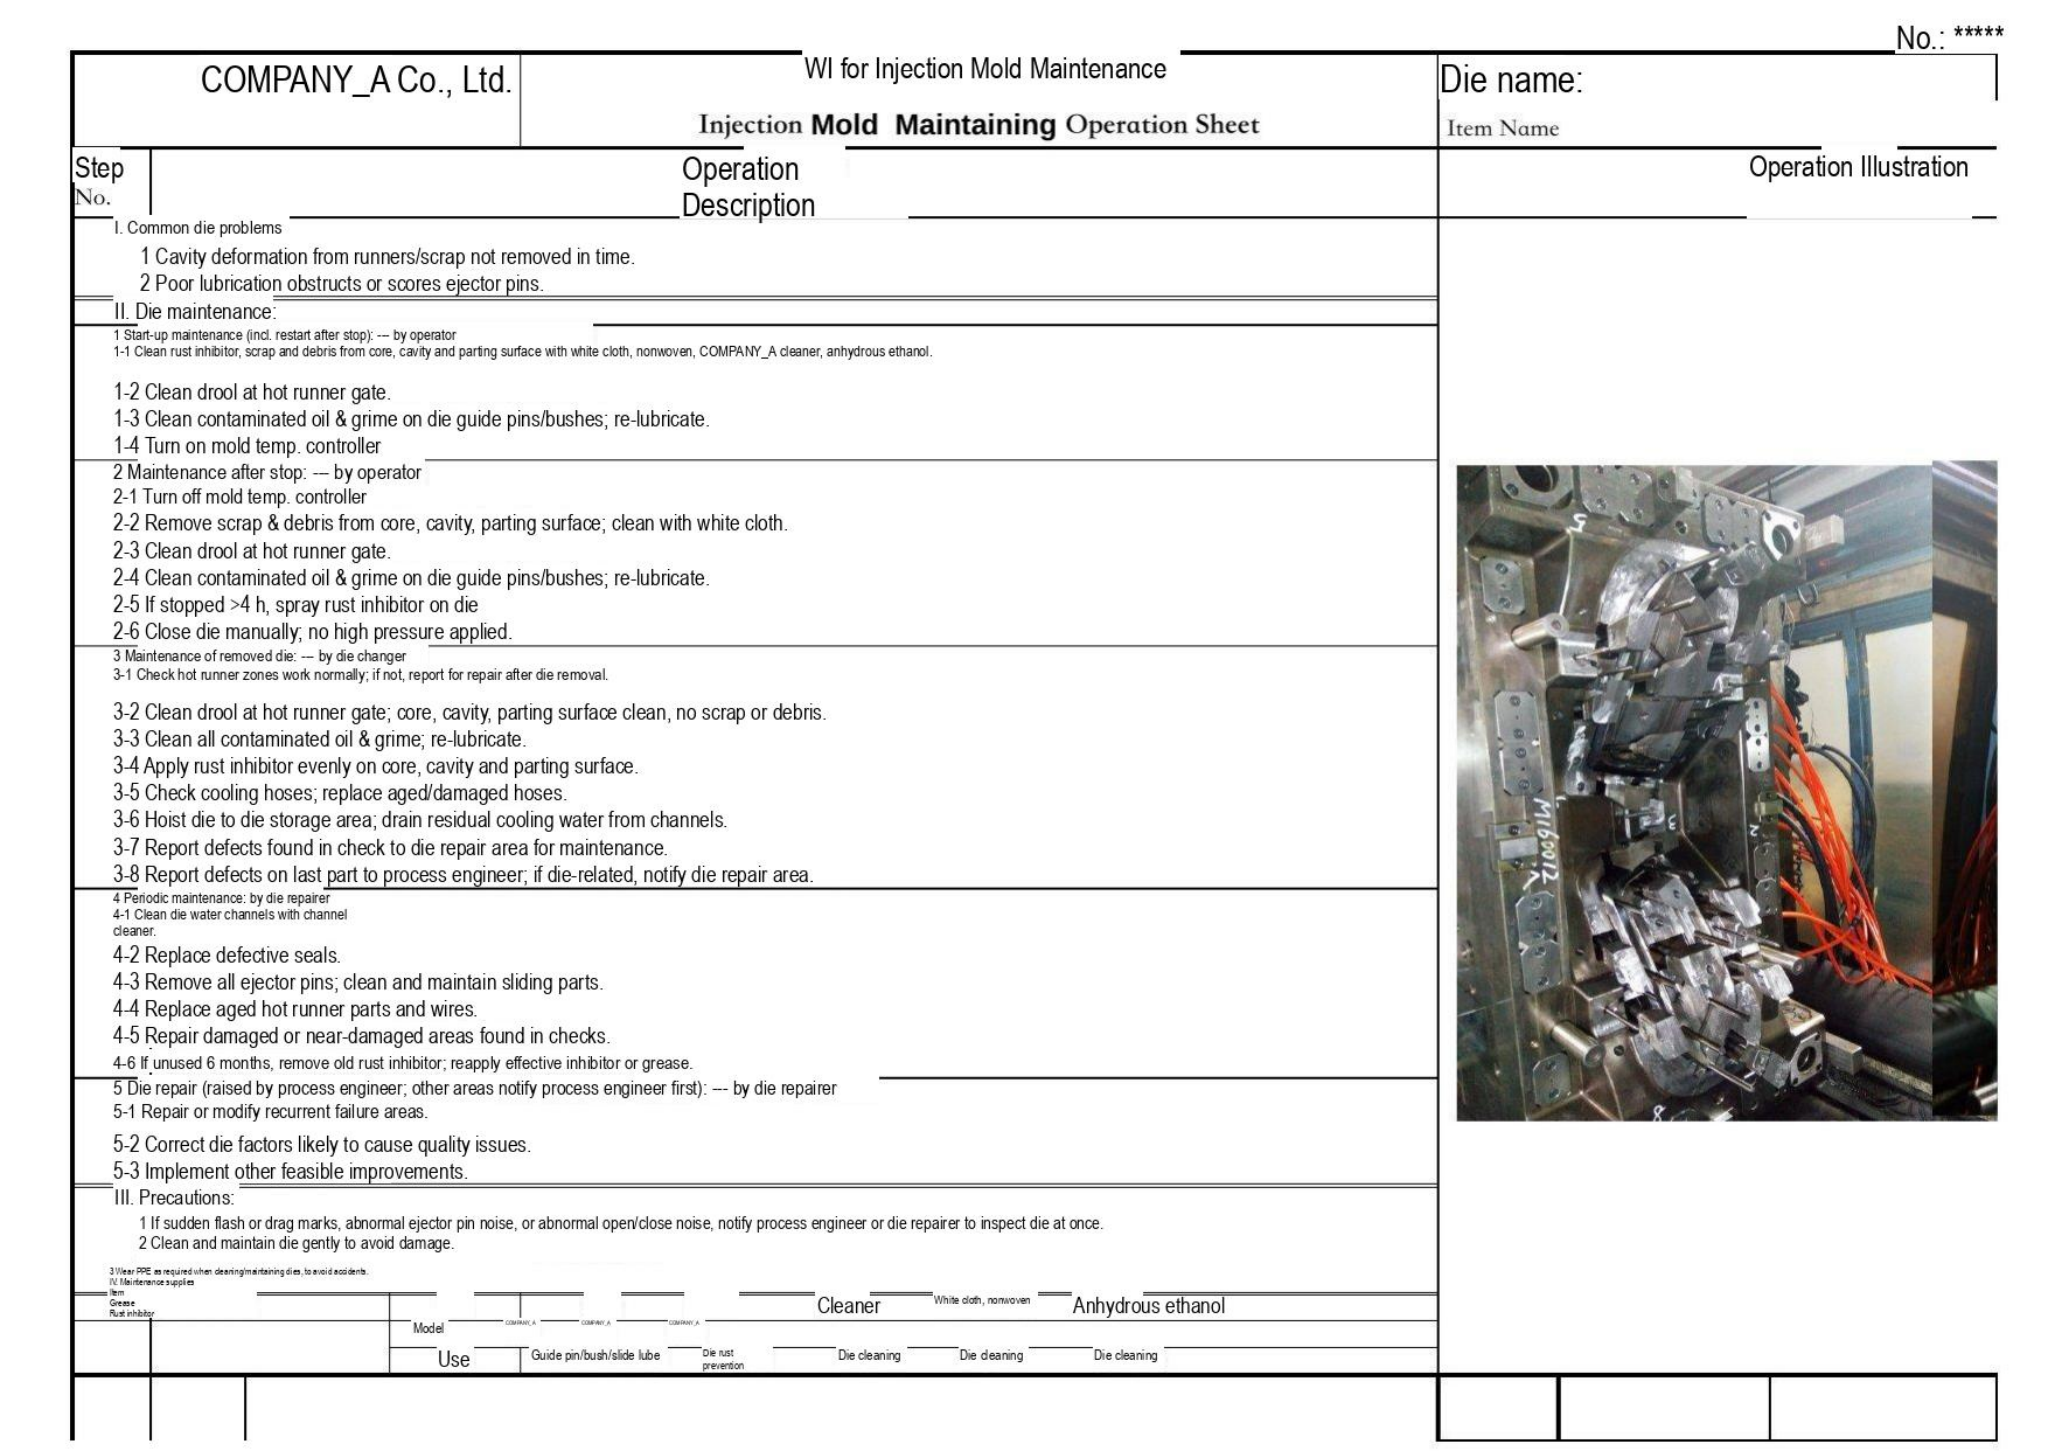No.: *****

COMPANY_A Co., Ltd.

WI for Injection Mold Maintenance

Injection Mold Maintaining Operation Sheet

Die name:

Item Name

Step No.

Operation Description

Operation Illustration

I. Common die problems

1 Cavity deformation from runners/scrap not removed in time.

2 Poor lubrication obstructs or scores ejector pins.

II. Die maintenance:

1 Start-up maintenance (incl. restart after stop): --- by operator

1-1 Clean rust inhibitor, scrap and debris from core, cavity and parting surface with white cloth, nonwoven, COMPANY_A cleaner, anhydrous ethanol.

1-2 Clean drool at hot runner gate.

1-3 Clean contaminated oil & grime on die guide pins/bushes; re-lubricate.

1-4 Turn on mold temp. controller

2 Maintenance after stop: --- by operator

2-1 Turn off mold temp. controller

2-2 Remove scrap & debris from core, cavity, parting surface; clean with white cloth.

2-3 Clean drool at hot runner gate.

2-4 Clean contaminated oil & grime on die guide pins/bushes; re-lubricate.

2-5 If stopped >4 h, spray rust inhibitor on die

2-6 Close die manually; no high pressure applied.

3 Maintenance of removed die: --- by die changer

3-1 Check hot runner zones work normally; if not, report for repair after die removal.

3-2 Clean drool at hot runner gate; core, cavity, parting surface clean, no scrap or debris.

3-3 Clean all contaminated oil & grime; re-lubricate.

3-4 Apply rust inhibitor evenly on core, cavity and parting surface.

3-5 Check cooling hoses; replace aged/damaged hoses.

3-6 Hoist die to die storage area; drain residual cooling water from channels.

3-7 Report defects found in check to die repair area for maintenance.

3-8 Report defects on last part to process engineer; if die-related, notify die repair area.

4 Periodic maintenance: by die repairer

4-1 Clean die water channels with channel cleaner.

4-2 Replace defective seals.

4-3 Remove all ejector pins; clean and maintain sliding parts.

4-4 Replace aged hot runner parts and wires.

4-5 Repair damaged or near-damaged areas found in checks.

4-6 If unused 6 months, remove old rust inhibitor; reapply effective inhibitor or grease.

5 Die repair (raised by process engineer; other areas notify process engineer first): --- by die repairer

5-1 Repair or modify recurrent failure areas.

5-2 Correct die factors likely to cause quality issues.

5-3 Implement other feasible improvements.

III. Precautions:

1 If sudden flash or drag marks, abnormal ejector pin noise, or abnormal open/close noise, notify process engineer or die repairer to inspect die at once.

2 Clean and maintain die gently to avoid damage.

3 Wear PPE as required when cleaning/maintaining dies, to avoid accidents.

IV. Maintenance supplies

| Item | Grease | Rust inhibitor | Cleaner | White cloth, nonwoven | Anhydrous ethanol |
|---|---|---|---|---|---|
| Model | COMPANY_A | COMPANY_A | COMPANY_A | | |
| Use | Guide pin/bush/slide lube | Die rust prevention | Die cleaning | Die cleaning | Die cleaning |

M160012
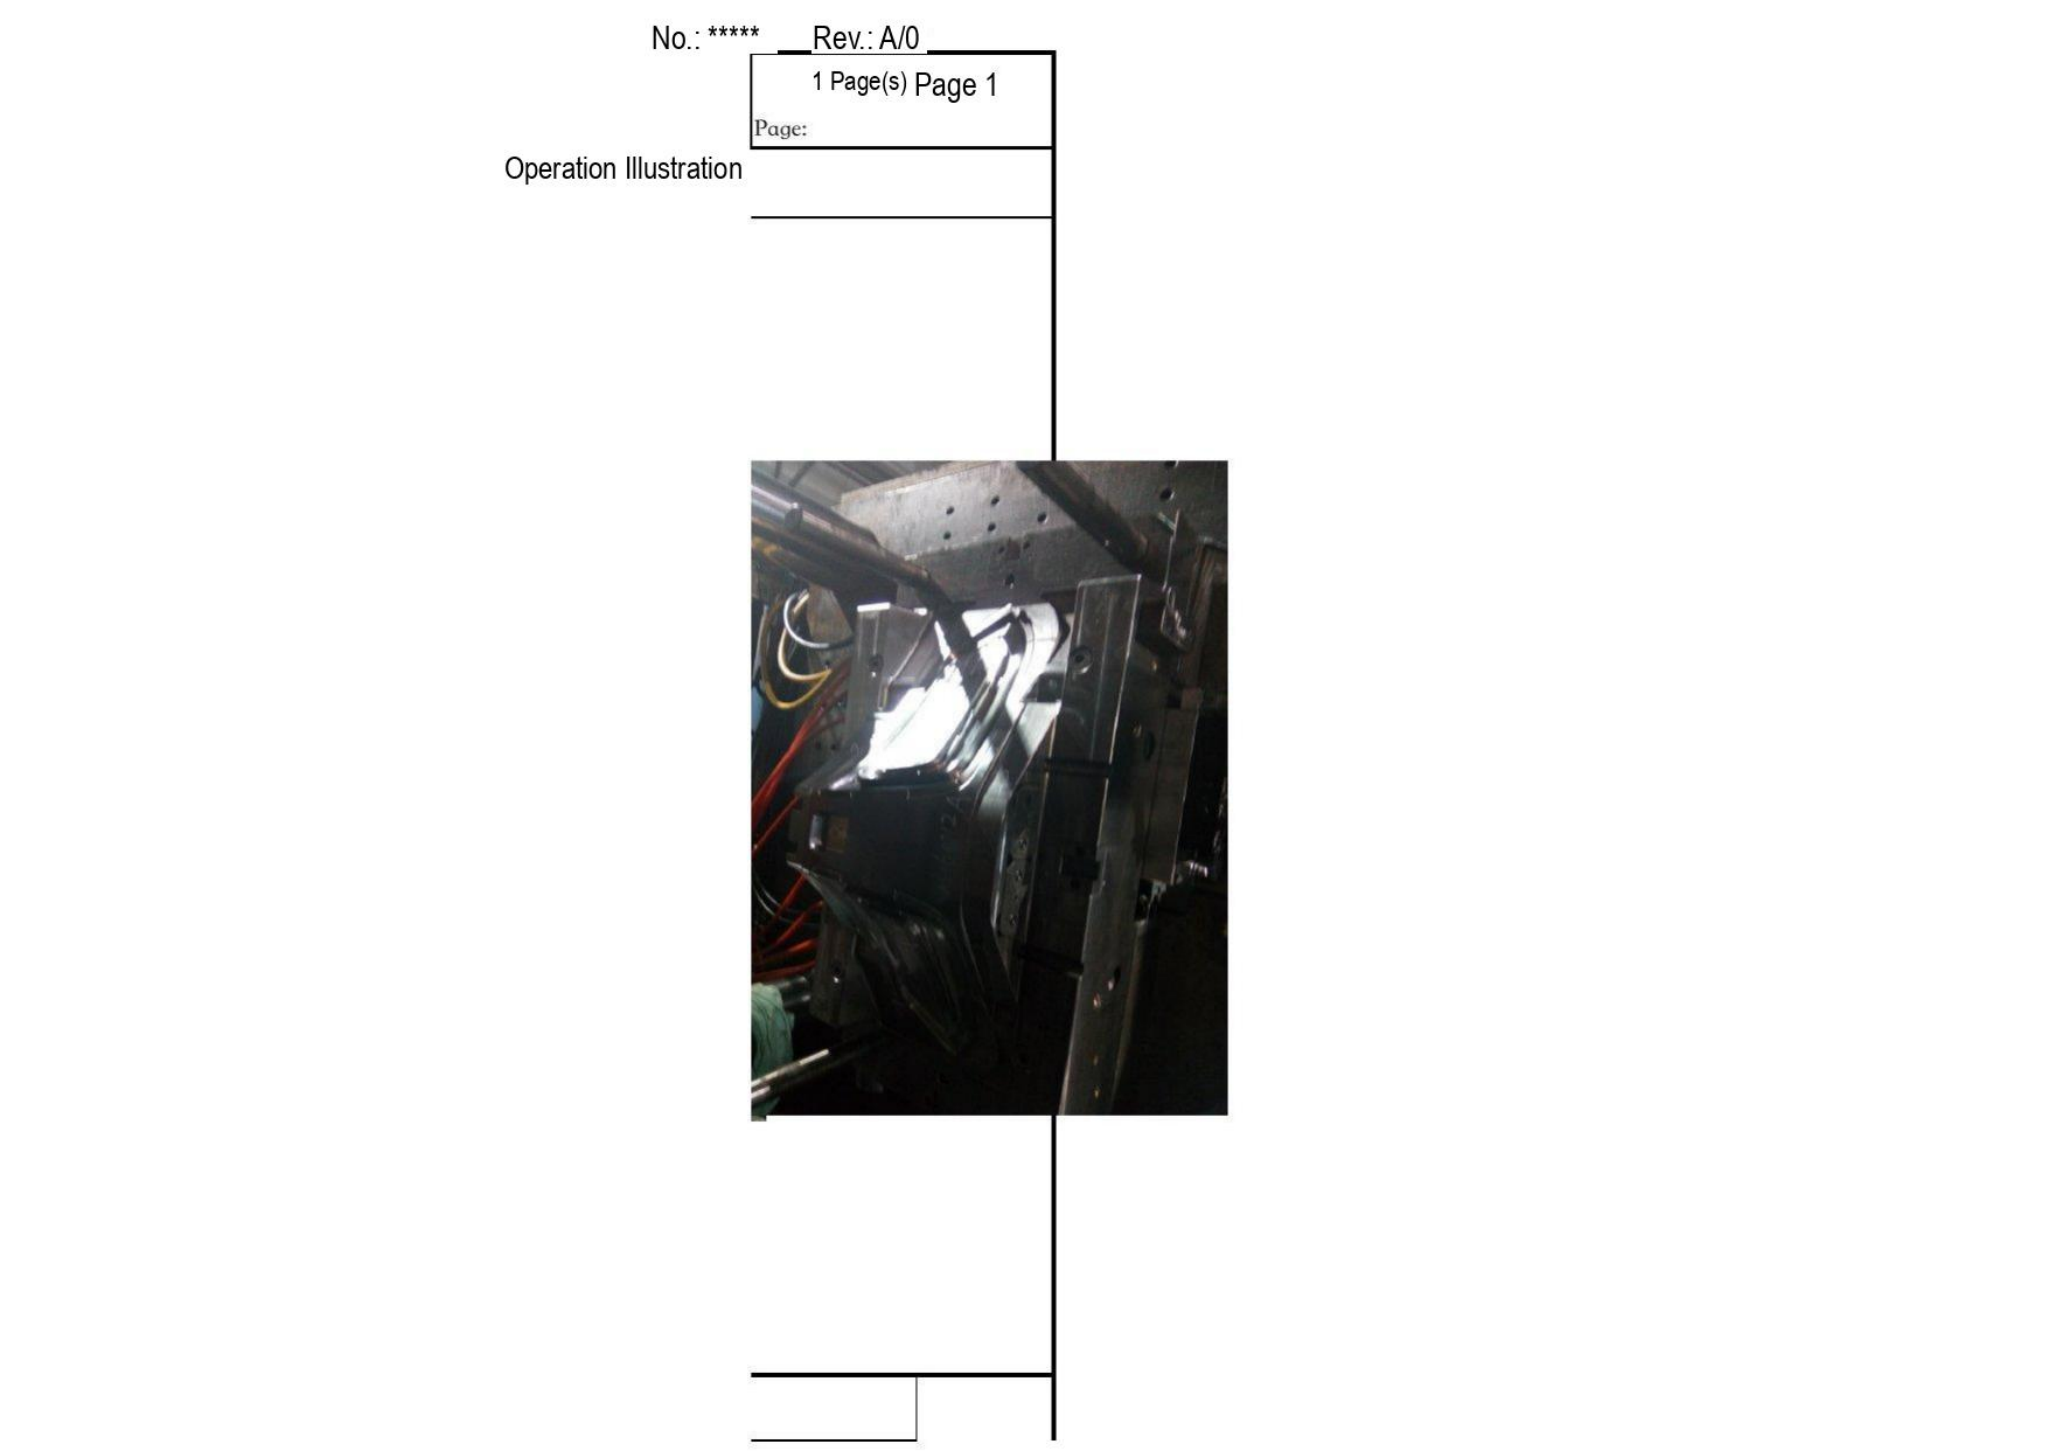No.: ***** Rev.: A/0

1 Page(s) Page 1

Page:

Operation Illustration